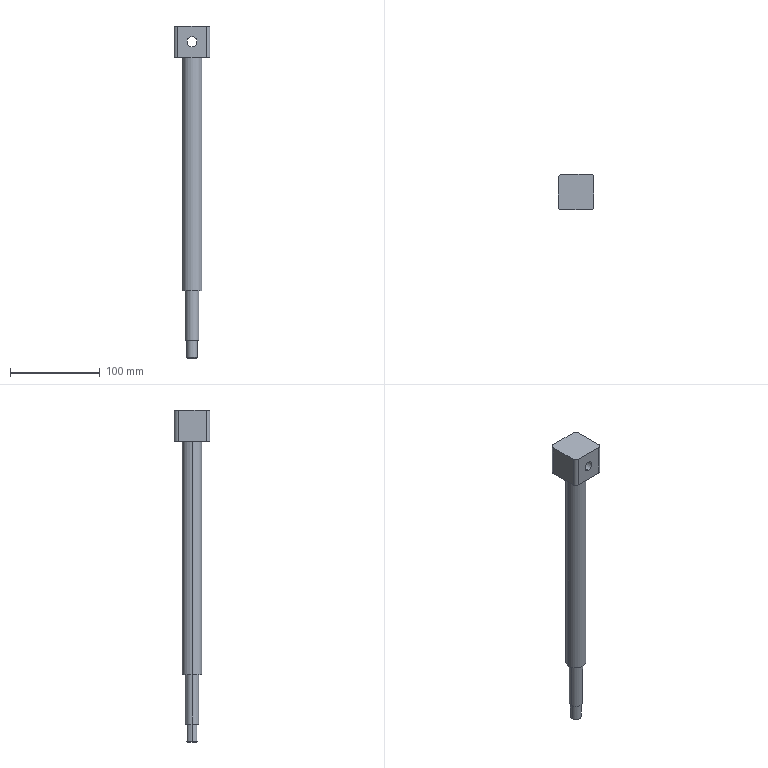Part | SolidWorks | features ICE 4, Chamfer 1, Extrusion 1 | 1 solid | 23 faces | box 40 x 40 x 370 mm | volume 162450 mm3 | cylinder 12 | plane 9 | cone 2 | commonest cylinder face diameters 7.977 x3 11 x2 12 x2 15 x2 22 x2 10 x1
STEP:
#1=CARTESIAN_POINT('',(-5.,0.,-352.5));
#2=VERTEX_POINT('',#1);
#3=CARTESIAN_POINT('',(5.,0.,-352.5));
#4=VERTEX_POINT('',#3);
#5=CARTESIAN_POINT('',(0.,0.,-352.5));
#6=DIRECTION('',(0.,0.,-1.));
#7=DIRECTION('',(-1.,0.,0.));
#8=AXIS2_PLACEMENT_3D('',#5,#6,#7);
#9=CIRCLE('',#8,5.);
#10=EDGE_CURVE('',#2,#4,#9,.T.);
#11=ORIENTED_EDGE('',*,*,#10,.F.);
#12=CARTESIAN_POINT('',(-6.,0.,-351.5));
#13=VERTEX_POINT('',#12);
#14=CARTESIAN_POINT('',(-5.,0.,-352.5));
#15=DIRECTION('',(-0.7071,0.,0.7071));
#16=VECTOR('',#15,1000.);
#17=LINE('',#14,#16);
#18=EDGE_CURVE('',#2,#13,#17,.T.);
#19=ORIENTED_EDGE('',*,*,#18,.T.);
#20=CARTESIAN_POINT('',(6.,0.,-351.5));
#21=VERTEX_POINT('',#20);
#22=CARTESIAN_POINT('',(0.,0.,-351.5));
#23=DIRECTION('',(0.,0.,1.));
#24=DIRECTION('',(-1.,0.,0.));
#25=AXIS2_PLACEMENT_3D('',#22,#23,#24);
#26=CIRCLE('',#25,6.);
#27=EDGE_CURVE('',#21,#13,#26,.T.);
#28=ORIENTED_EDGE('',*,*,#27,.F.);
#29=CARTESIAN_POINT('',(5.,0.,-352.5));
#30=DIRECTION('',(0.7071,0.,0.7071));
#31=VECTOR('',#30,1000.);
#32=LINE('',#29,#31);
#33=EDGE_CURVE('',#4,#21,#32,.T.);
#34=ORIENTED_EDGE('',*,*,#33,.F.);
#35=EDGE_LOOP('',(#11,#19,#28,#34));
#36=FACE_OUTER_BOUND('',#35,.T.);
#37=CARTESIAN_POINT('',(0.,0.,-352.5));
#38=DIRECTION('',(0.,0.,1.));
#39=DIRECTION('',(1.,0.,0.));
#40=AXIS2_PLACEMENT_3D('',#37,#38,#39);
#41=CONICAL_SURFACE('',#40,5.,0.7854);
#42=ADVANCED_FACE('',(#36),#41,.T.);
#43=ORIENTED_EDGE('',*,*,#27,.T.);
#44=CARTESIAN_POINT('',(-6.,0.,-332.5));
#45=VERTEX_POINT('',#44);
#46=CARTESIAN_POINT('',(-6.,0.,-352.5));
#47=DIRECTION('',(0.,0.,1.));
#48=VECTOR('',#47,1000.);
#49=LINE('',#46,#48);
#50=EDGE_CURVE('',#13,#45,#49,.T.);
#51=ORIENTED_EDGE('',*,*,#50,.T.);
#52=CARTESIAN_POINT('',(6.,0.,-332.5));
#53=VERTEX_POINT('',#52);
#54=CARTESIAN_POINT('',(0.,0.,-332.5));
#55=DIRECTION('',(0.,0.,-1.));
#56=DIRECTION('',(-1.,0.,0.));
#57=AXIS2_PLACEMENT_3D('',#54,#55,#56);
#58=CIRCLE('',#57,6.);
#59=EDGE_CURVE('',#45,#53,#58,.T.);
#60=ORIENTED_EDGE('',*,*,#59,.T.);
#61=CARTESIAN_POINT('',(6.,0.,-352.5));
#62=DIRECTION('',(0.,0.,1.));
#63=VECTOR('',#62,1000.);
#64=LINE('',#61,#63);
#65=EDGE_CURVE('',#21,#53,#64,.T.);
#66=ORIENTED_EDGE('',*,*,#65,.F.);
#67=EDGE_LOOP('',(#43,#51,#60,#66));
#68=FACE_OUTER_BOUND('',#67,.T.);
#69=CARTESIAN_POINT('',(0.,0.,-352.5));
#70=DIRECTION('',(0.,0.,1.));
#71=DIRECTION('',(1.,0.,0.));
#72=AXIS2_PLACEMENT_3D('',#69,#70,#71);
#73=CYLINDRICAL_SURFACE('',#72,6.);
#74=ADVANCED_FACE('',(#68),#73,.T.);
#75=CARTESIAN_POINT('',(-7.5,0.,-332.5));
#76=VERTEX_POINT('',#75);
#77=CARTESIAN_POINT('',(7.5,0.,-332.5));
#78=VERTEX_POINT('',#77);
#79=CARTESIAN_POINT('',(0.,0.,-332.5));
#80=DIRECTION('',(0.,0.,-1.));
#81=DIRECTION('',(-1.,0.,0.));
#82=AXIS2_PLACEMENT_3D('',#79,#80,#81);
#83=CIRCLE('',#82,7.5);
#84=EDGE_CURVE('',#76,#78,#83,.T.);
#85=ORIENTED_EDGE('',*,*,#84,.F.);
#86=CARTESIAN_POINT('',(-7.5,0.,-277.5));
#87=VERTEX_POINT('',#86);
#88=CARTESIAN_POINT('',(-7.5,0.,-332.5));
#89=DIRECTION('',(0.,0.,1.));
#90=VECTOR('',#89,1000.);
#91=LINE('',#88,#90);
#92=EDGE_CURVE('',#76,#87,#91,.T.);
#93=ORIENTED_EDGE('',*,*,#92,.T.);
#94=CARTESIAN_POINT('',(7.5,0.,-277.5));
#95=VERTEX_POINT('',#94);
#96=CARTESIAN_POINT('',(0.,0.,-277.5));
#97=DIRECTION('',(0.,0.,-1.));
#98=DIRECTION('',(-1.,0.,0.));
#99=AXIS2_PLACEMENT_3D('',#96,#97,#98);
#100=CIRCLE('',#99,7.5);
#101=EDGE_CURVE('',#87,#95,#100,.T.);
#102=ORIENTED_EDGE('',*,*,#101,.T.);
#103=CARTESIAN_POINT('',(7.5,0.,-332.5));
#104=DIRECTION('',(0.,0.,1.));
#105=VECTOR('',#104,1000.);
#106=LINE('',#103,#105);
#107=EDGE_CURVE('',#78,#95,#106,.T.);
#108=ORIENTED_EDGE('',*,*,#107,.F.);
#109=EDGE_LOOP('',(#85,#93,#102,#108));
#110=FACE_OUTER_BOUND('',#109,.T.);
#111=CARTESIAN_POINT('',(0.,0.,-332.5));
#112=DIRECTION('',(0.,0.,1.));
#113=DIRECTION('',(1.,0.,0.));
#114=AXIS2_PLACEMENT_3D('',#111,#112,#113);
#115=CYLINDRICAL_SURFACE('',#114,7.5);
#116=ADVANCED_FACE('',(#110),#115,.T.);
#117=CARTESIAN_POINT('',(-11.,0.,-277.5));
#118=VERTEX_POINT('',#117);
#119=CARTESIAN_POINT('',(11.,0.,-277.5));
#120=VERTEX_POINT('',#119);
#121=CARTESIAN_POINT('',(0.,0.,-277.5));
#122=DIRECTION('',(0.,0.,-1.));
#123=DIRECTION('',(-1.,0.,0.));
#124=AXIS2_PLACEMENT_3D('',#121,#122,#123);
#125=CIRCLE('',#124,11.);
#126=EDGE_CURVE('',#118,#120,#125,.T.);
#127=ORIENTED_EDGE('',*,*,#126,.F.);
#128=CARTESIAN_POINT('',(-11.,0.,-17.5));
#129=VERTEX_POINT('',#128);
#130=CARTESIAN_POINT('',(-11.,0.,-277.5));
#131=DIRECTION('',(0.,0.,1.));
#132=VECTOR('',#131,1000.);
#133=LINE('',#130,#132);
#134=EDGE_CURVE('',#118,#129,#133,.T.);
#135=ORIENTED_EDGE('',*,*,#134,.T.);
#136=CARTESIAN_POINT('',(11.,0.,-17.5));
#137=VERTEX_POINT('',#136);
#138=CARTESIAN_POINT('',(0.,0.,-17.5));
#139=DIRECTION('',(0.,0.,-1.));
#140=DIRECTION('',(-1.,0.,0.));
#141=AXIS2_PLACEMENT_3D('',#138,#139,#140);
#142=CIRCLE('',#141,11.);
#143=EDGE_CURVE('',#129,#137,#142,.T.);
#144=ORIENTED_EDGE('',*,*,#143,.T.);
#145=CARTESIAN_POINT('',(11.,0.,-277.5));
#146=DIRECTION('',(0.,0.,1.));
#147=VECTOR('',#146,1000.);
#148=LINE('',#145,#147);
#149=EDGE_CURVE('',#120,#137,#148,.T.);
#150=ORIENTED_EDGE('',*,*,#149,.F.);
#151=EDGE_LOOP('',(#127,#135,#144,#150));
#152=FACE_OUTER_BOUND('',#151,.T.);
#153=CARTESIAN_POINT('',(0.,0.,-277.5));
#154=DIRECTION('',(0.,0.,1.));
#155=DIRECTION('',(1.,0.,0.));
#156=AXIS2_PLACEMENT_3D('',#153,#154,#155);
#157=CYLINDRICAL_SURFACE('',#156,11.);
#158=ADVANCED_FACE('',(#152),#157,.T.);
#159=CARTESIAN_POINT('',(0.,-20.,-5.5));
#160=VERTEX_POINT('',#159);
#161=CARTESIAN_POINT('',(0.,-20.,5.5));
#162=VERTEX_POINT('',#161);
#163=CARTESIAN_POINT('',(0.,-20.,0.));
#164=DIRECTION('',(0.,1.,0.));
#165=DIRECTION('',(0.,0.,1.));
#166=AXIS2_PLACEMENT_3D('',#163,#164,#165);
#167=CIRCLE('',#166,5.5);
#168=EDGE_CURVE('',#160,#162,#167,.T.);
#169=ORIENTED_EDGE('',*,*,#168,.F.);
#170=CARTESIAN_POINT('',(0.,20.,-5.5));
#171=VERTEX_POINT('',#170);
#172=CARTESIAN_POINT('',(0.,-34.,-5.5));
#173=DIRECTION('',(0.,1.,0.));
#174=VECTOR('',#173,1000.);
#175=LINE('',#172,#174);
#176=EDGE_CURVE('',#160,#171,#175,.T.);
#177=ORIENTED_EDGE('',*,*,#176,.T.);
#178=CARTESIAN_POINT('',(0.,20.,5.5));
#179=VERTEX_POINT('',#178);
#180=CARTESIAN_POINT('',(0.,20.,0.));
#181=DIRECTION('',(0.,1.,0.));
#182=DIRECTION('',(0.,0.,1.));
#183=AXIS2_PLACEMENT_3D('',#180,#181,#182);
#184=CIRCLE('',#183,5.5);
#185=EDGE_CURVE('',#171,#179,#184,.T.);
#186=ORIENTED_EDGE('',*,*,#185,.T.);
#187=CARTESIAN_POINT('',(0.,-34.,5.5));
#188=DIRECTION('',(0.,1.,0.));
#189=VECTOR('',#188,1000.);
#190=LINE('',#187,#189);
#191=EDGE_CURVE('',#162,#179,#190,.T.);
#192=ORIENTED_EDGE('',*,*,#191,.F.);
#193=EDGE_LOOP('',(#169,#177,#186,#192));
#194=FACE_OUTER_BOUND('',#193,.T.);
#195=CARTESIAN_POINT('',(0.,-34.,0.));
#196=DIRECTION('',(0.,1.,0.));
#197=DIRECTION('',(0.,0.,1.));
#198=AXIS2_PLACEMENT_3D('',#195,#196,#197);
#199=CYLINDRICAL_SURFACE('',#198,5.5);
#200=ADVANCED_FACE('',(#194),#199,.F.);
#201=CARTESIAN_POINT('',(0.,0.,-332.5));
#202=DIRECTION('',(0.,0.,-1.));
#203=DIRECTION('',(-1.,0.,0.));
#204=AXIS2_PLACEMENT_3D('',#201,#202,#203);
#205=CIRCLE('',#204,7.5);
#206=EDGE_CURVE('',#78,#76,#205,.T.);
#207=ORIENTED_EDGE('',*,*,#206,.T.);
#208=ORIENTED_EDGE('',*,*,#84,.T.);
#209=EDGE_LOOP('',(#207,#208));
#210=FACE_OUTER_BOUND('',#209,.T.);
#211=CARTESIAN_POINT('',(0.,0.,-332.5));
#212=DIRECTION('',(0.,0.,-1.));
#213=DIRECTION('',(-1.,0.,0.));
#214=AXIS2_PLACEMENT_3D('',#211,#212,#213);
#215=CIRCLE('',#214,6.);
#216=EDGE_CURVE('',#53,#45,#215,.T.);
#217=ORIENTED_EDGE('',*,*,#216,.F.);
#218=ORIENTED_EDGE('',*,*,#59,.F.);
#219=EDGE_LOOP('',(#217,#218));
#220=FACE_BOUND('',#219,.T.);
#221=CARTESIAN_POINT('',(0.,0.,-332.5));
#222=DIRECTION('',(0.,0.,-1.));
#223=DIRECTION('',(-1.,0.,0.));
#224=AXIS2_PLACEMENT_3D('',#221,#222,#223);
#225=PLANE('',#224);
#226=ADVANCED_FACE('',(#210,#220),#225,.T.);
#227=CARTESIAN_POINT('',(0.,0.,-277.5));
#228=DIRECTION('',(0.,0.,-1.));
#229=DIRECTION('',(-1.,0.,0.));
#230=AXIS2_PLACEMENT_3D('',#227,#228,#229);
#231=CIRCLE('',#230,11.);
#232=EDGE_CURVE('',#120,#118,#231,.T.);
#233=ORIENTED_EDGE('',*,*,#232,.T.);
#234=ORIENTED_EDGE('',*,*,#126,.T.);
#235=EDGE_LOOP('',(#233,#234));
#236=FACE_OUTER_BOUND('',#235,.T.);
#237=CARTESIAN_POINT('',(0.,0.,-277.5));
#238=DIRECTION('',(0.,0.,-1.));
#239=DIRECTION('',(-1.,0.,0.));
#240=AXIS2_PLACEMENT_3D('',#237,#238,#239);
#241=CIRCLE('',#240,7.5);
#242=EDGE_CURVE('',#95,#87,#241,.T.);
#243=ORIENTED_EDGE('',*,*,#242,.F.);
#244=ORIENTED_EDGE('',*,*,#101,.F.);
#245=EDGE_LOOP('',(#243,#244));
#246=FACE_BOUND('',#245,.T.);
#247=CARTESIAN_POINT('',(0.,0.,-277.5));
#248=DIRECTION('',(0.,0.,-1.));
#249=DIRECTION('',(-1.,0.,0.));
#250=AXIS2_PLACEMENT_3D('',#247,#248,#249);
#251=PLANE('',#250);
#252=ADVANCED_FACE('',(#236,#246),#251,.T.);
#253=CARTESIAN_POINT('',(-15.,20.,-17.5));
#254=VERTEX_POINT('',#253);
#255=CARTESIAN_POINT('',(-20.,15.,-17.5));
#256=VERTEX_POINT('',#255);
#257=CARTESIAN_POINT('',(-15.,15.,-17.5));
#258=DIRECTION('',(0.,0.,1.));
#259=DIRECTION('',(-1.,0.,0.));
#260=AXIS2_PLACEMENT_3D('',#257,#258,#259);
#261=CIRCLE('',#260,5.);
#262=EDGE_CURVE('',#254,#256,#261,.T.);
#263=ORIENTED_EDGE('',*,*,#262,.F.);
#264=CARTESIAN_POINT('',(16.011,20.,-17.5));
#265=VERTEX_POINT('',#264);
#266=CARTESIAN_POINT('',(-15.,20.,-17.5));
#267=DIRECTION('',(-1.,0.,0.));
#268=VECTOR('',#267,1000.);
#269=LINE('',#266,#268);
#270=EDGE_CURVE('',#265,#254,#269,.T.);
#271=ORIENTED_EDGE('',*,*,#270,.F.);
#272=CARTESIAN_POINT('',(20.,16.011,-17.5));
#273=VERTEX_POINT('',#272);
#274=CARTESIAN_POINT('',(16.011,16.011,-17.5));
#275=DIRECTION('',(0.,0.,1.));
#276=DIRECTION('',(1.,0.,0.));
#277=AXIS2_PLACEMENT_3D('',#274,#275,#276);
#278=CIRCLE('',#277,3.989);
#279=EDGE_CURVE('',#273,#265,#278,.T.);
#280=ORIENTED_EDGE('',*,*,#279,.F.);
#281=CARTESIAN_POINT('',(20.,-16.011,-17.5));
#282=VERTEX_POINT('',#281);
#283=CARTESIAN_POINT('',(20.,16.011,-17.5));
#284=DIRECTION('',(0.,1.,0.));
#285=VECTOR('',#284,1000.);
#286=LINE('',#283,#285);
#287=EDGE_CURVE('',#282,#273,#286,.T.);
#288=ORIENTED_EDGE('',*,*,#287,.F.);
#289=CARTESIAN_POINT('',(16.011,-20.,-17.5));
#290=VERTEX_POINT('',#289);
#291=CARTESIAN_POINT('',(16.011,-16.011,-17.5));
#292=DIRECTION('',(0.,0.,1.));
#293=DIRECTION('',(1.,0.,0.));
#294=AXIS2_PLACEMENT_3D('',#291,#292,#293);
#295=CIRCLE('',#294,3.989);
#296=EDGE_CURVE('',#290,#282,#295,.T.);
#297=ORIENTED_EDGE('',*,*,#296,.F.);
#298=CARTESIAN_POINT('',(-16.011,-20.,-17.5));
#299=VERTEX_POINT('',#298);
#300=CARTESIAN_POINT('',(-16.011,-20.,-17.5));
#301=DIRECTION('',(1.,0.,0.));
#302=VECTOR('',#301,1000.);
#303=LINE('',#300,#302);
#304=EDGE_CURVE('',#299,#290,#303,.T.);
#305=ORIENTED_EDGE('',*,*,#304,.F.);
#306=CARTESIAN_POINT('',(-20.,-16.011,-17.5));
#307=VERTEX_POINT('',#306);
#308=CARTESIAN_POINT('',(-16.011,-16.011,-17.5));
#309=DIRECTION('',(0.,0.,1.));
#310=DIRECTION('',(-1.,0.,0.));
#311=AXIS2_PLACEMENT_3D('',#308,#309,#310);
#312=CIRCLE('',#311,3.989);
#313=EDGE_CURVE('',#307,#299,#312,.T.);
#314=ORIENTED_EDGE('',*,*,#313,.F.);
#315=CARTESIAN_POINT('',(-20.,15.,-17.5));
#316=DIRECTION('',(0.,-1.,0.));
#317=VECTOR('',#316,1000.);
#318=LINE('',#315,#317);
#319=EDGE_CURVE('',#256,#307,#318,.T.);
#320=ORIENTED_EDGE('',*,*,#319,.F.);
#321=EDGE_LOOP('',(#263,#271,#280,#288,#297,#305,#314,#320));
#322=FACE_OUTER_BOUND('',#321,.T.);
#323=CARTESIAN_POINT('',(0.,0.,-17.5));
#324=DIRECTION('',(0.,0.,-1.));
#325=DIRECTION('',(-1.,0.,0.));
#326=AXIS2_PLACEMENT_3D('',#323,#324,#325);
#327=CIRCLE('',#326,11.);
#328=EDGE_CURVE('',#137,#129,#327,.T.);
#329=ORIENTED_EDGE('',*,*,#328,.F.);
#330=ORIENTED_EDGE('',*,*,#143,.F.);
#331=EDGE_LOOP('',(#329,#330));
#332=FACE_BOUND('',#331,.T.);
#333=CARTESIAN_POINT('',(-15.,15.,-17.5));
#334=DIRECTION('',(0.,0.,-1.));
#335=DIRECTION('',(-1.,0.,0.));
#336=AXIS2_PLACEMENT_3D('',#333,#334,#335);
#337=PLANE('',#336);
#338=ADVANCED_FACE('',(#322,#332),#337,.T.);
#339=ORIENTED_EDGE('',*,*,#262,.T.);
#340=CARTESIAN_POINT('',(-20.,15.,17.5));
#341=VERTEX_POINT('',#340);
#342=CARTESIAN_POINT('',(-20.,15.,17.5));
#343=DIRECTION('',(0.,0.,-1.));
#344=VECTOR('',#343,1000.);
#345=LINE('',#342,#344);
#346=EDGE_CURVE('',#341,#256,#345,.T.);
#347=ORIENTED_EDGE('',*,*,#346,.F.);
#348=CARTESIAN_POINT('',(-15.,20.,17.5));
#349=VERTEX_POINT('',#348);
#350=CARTESIAN_POINT('',(-15.,15.,17.5));
#351=DIRECTION('',(0.,0.,1.));
#352=DIRECTION('',(-1.,0.,0.));
#353=AXIS2_PLACEMENT_3D('',#350,#351,#352);
#354=CIRCLE('',#353,5.);
#355=EDGE_CURVE('',#349,#341,#354,.T.);
#356=ORIENTED_EDGE('',*,*,#355,.F.);
#357=CARTESIAN_POINT('',(-15.,20.,17.5));
#358=DIRECTION('',(0.,0.,-1.));
#359=VECTOR('',#358,1000.);
#360=LINE('',#357,#359);
#361=EDGE_CURVE('',#349,#254,#360,.T.);
#362=ORIENTED_EDGE('',*,*,#361,.T.);
#363=EDGE_LOOP('',(#339,#347,#356,#362));
#364=FACE_OUTER_BOUND('',#363,.T.);
#365=CARTESIAN_POINT('',(-15.,15.,17.5));
#366=DIRECTION('',(0.,0.,-1.));
#367=DIRECTION('',(-1.,0.,0.));
#368=AXIS2_PLACEMENT_3D('',#365,#366,#367);
#369=CYLINDRICAL_SURFACE('',#368,5.);
#370=ADVANCED_FACE('',(#364),#369,.T.);
#371=ORIENTED_EDGE('',*,*,#319,.T.);
#372=CARTESIAN_POINT('',(-20.,-16.011,17.5));
#373=VERTEX_POINT('',#372);
#374=CARTESIAN_POINT('',(-20.,-16.011,17.5));
#375=DIRECTION('',(0.,0.,-1.));
#376=VECTOR('',#375,1000.);
#377=LINE('',#374,#376);
#378=EDGE_CURVE('',#373,#307,#377,.T.);
#379=ORIENTED_EDGE('',*,*,#378,.F.);
#380=CARTESIAN_POINT('',(-20.,15.,17.5));
#381=DIRECTION('',(0.,-1.,0.));
#382=VECTOR('',#381,1000.);
#383=LINE('',#380,#382);
#384=EDGE_CURVE('',#341,#373,#383,.T.);
#385=ORIENTED_EDGE('',*,*,#384,.F.);
#386=ORIENTED_EDGE('',*,*,#346,.T.);
#387=EDGE_LOOP('',(#371,#379,#385,#386));
#388=FACE_OUTER_BOUND('',#387,.T.);
#389=CARTESIAN_POINT('',(-20.,15.,17.5));
#390=DIRECTION('',(1.,0.,0.));
#391=DIRECTION('',(0.,1.,0.));
#392=AXIS2_PLACEMENT_3D('',#389,#390,#391);
#393=PLANE('',#392);
#394=ADVANCED_FACE('',(#388),#393,.F.);
#395=ORIENTED_EDGE('',*,*,#313,.T.);
#396=CARTESIAN_POINT('',(-16.011,-20.,17.5));
#397=VERTEX_POINT('',#396);
#398=CARTESIAN_POINT('',(-16.011,-20.,17.5));
#399=DIRECTION('',(0.,0.,-1.));
#400=VECTOR('',#399,1000.);
#401=LINE('',#398,#400);
#402=EDGE_CURVE('',#397,#299,#401,.T.);
#403=ORIENTED_EDGE('',*,*,#402,.F.);
#404=CARTESIAN_POINT('',(-16.011,-16.011,17.5));
#405=DIRECTION('',(0.,0.,1.));
#406=DIRECTION('',(-1.,0.,0.));
#407=AXIS2_PLACEMENT_3D('',#404,#405,#406);
#408=CIRCLE('',#407,3.989);
#409=EDGE_CURVE('',#373,#397,#408,.T.);
#410=ORIENTED_EDGE('',*,*,#409,.F.);
#411=ORIENTED_EDGE('',*,*,#378,.T.);
#412=EDGE_LOOP('',(#395,#403,#410,#411));
#413=FACE_OUTER_BOUND('',#412,.T.);
#414=CARTESIAN_POINT('',(-16.011,-16.011,17.5));
#415=DIRECTION('',(0.,0.,-1.));
#416=DIRECTION('',(-1.,0.,0.));
#417=AXIS2_PLACEMENT_3D('',#414,#415,#416);
#418=CYLINDRICAL_SURFACE('',#417,3.989);
#419=ADVANCED_FACE('',(#413),#418,.T.);
#420=CARTESIAN_POINT('',(0.,-20.,0.));
#421=DIRECTION('',(0.,1.,0.));
#422=DIRECTION('',(0.,0.,1.));
#423=AXIS2_PLACEMENT_3D('',#420,#421,#422);
#424=CIRCLE('',#423,5.5);
#425=EDGE_CURVE('',#162,#160,#424,.T.);
#426=ORIENTED_EDGE('',*,*,#425,.T.);
#427=ORIENTED_EDGE('',*,*,#168,.T.);
#428=EDGE_LOOP('',(#426,#427));
#429=FACE_BOUND('',#428,.T.);
#430=ORIENTED_EDGE('',*,*,#304,.T.);
#431=CARTESIAN_POINT('',(16.011,-20.,17.5));
#432=VERTEX_POINT('',#431);
#433=CARTESIAN_POINT('',(16.011,-20.,17.5));
#434=DIRECTION('',(0.,0.,-1.));
#435=VECTOR('',#434,1000.);
#436=LINE('',#433,#435);
#437=EDGE_CURVE('',#432,#290,#436,.T.);
#438=ORIENTED_EDGE('',*,*,#437,.F.);
#439=CARTESIAN_POINT('',(-16.011,-20.,17.5));
#440=DIRECTION('',(1.,0.,0.));
#441=VECTOR('',#440,1000.);
#442=LINE('',#439,#441);
#443=EDGE_CURVE('',#397,#432,#442,.T.);
#444=ORIENTED_EDGE('',*,*,#443,.F.);
#445=ORIENTED_EDGE('',*,*,#402,.T.);
#446=EDGE_LOOP('',(#430,#438,#444,#445));
#447=FACE_OUTER_BOUND('',#446,.T.);
#448=CARTESIAN_POINT('',(-16.011,-20.,17.5));
#449=DIRECTION('',(0.,1.,0.));
#450=DIRECTION('',(0.,0.,1.));
#451=AXIS2_PLACEMENT_3D('',#448,#449,#450);
#452=PLANE('',#451);
#453=ADVANCED_FACE('',(#429,#447),#452,.F.);
#454=ORIENTED_EDGE('',*,*,#296,.T.);
#455=CARTESIAN_POINT('',(20.,-16.011,17.5));
#456=VERTEX_POINT('',#455);
#457=CARTESIAN_POINT('',(20.,-16.011,17.5));
#458=DIRECTION('',(0.,0.,-1.));
#459=VECTOR('',#458,1000.);
#460=LINE('',#457,#459);
#461=EDGE_CURVE('',#456,#282,#460,.T.);
#462=ORIENTED_EDGE('',*,*,#461,.F.);
#463=CARTESIAN_POINT('',(16.011,-16.011,17.5));
#464=DIRECTION('',(0.,0.,1.));
#465=DIRECTION('',(1.,0.,0.));
#466=AXIS2_PLACEMENT_3D('',#463,#464,#465);
#467=CIRCLE('',#466,3.989);
#468=EDGE_CURVE('',#432,#456,#467,.T.);
#469=ORIENTED_EDGE('',*,*,#468,.F.);
#470=ORIENTED_EDGE('',*,*,#437,.T.);
#471=EDGE_LOOP('',(#454,#462,#469,#470));
#472=FACE_OUTER_BOUND('',#471,.T.);
#473=CARTESIAN_POINT('',(16.011,-16.011,17.5));
#474=DIRECTION('',(0.,0.,-1.));
#475=DIRECTION('',(-1.,0.,0.));
#476=AXIS2_PLACEMENT_3D('',#473,#474,#475);
#477=CYLINDRICAL_SURFACE('',#476,3.989);
#478=ADVANCED_FACE('',(#472),#477,.T.);
#479=ORIENTED_EDGE('',*,*,#287,.T.);
#480=CARTESIAN_POINT('',(20.,16.011,17.5));
#481=VERTEX_POINT('',#480);
#482=CARTESIAN_POINT('',(20.,16.011,17.5));
#483=DIRECTION('',(0.,0.,-1.));
#484=VECTOR('',#483,1000.);
#485=LINE('',#482,#484);
#486=EDGE_CURVE('',#481,#273,#485,.T.);
#487=ORIENTED_EDGE('',*,*,#486,.F.);
#488=CARTESIAN_POINT('',(20.,16.011,17.5));
#489=DIRECTION('',(0.,1.,0.));
#490=VECTOR('',#489,1000.);
#491=LINE('',#488,#490);
#492=EDGE_CURVE('',#456,#481,#491,.T.);
#493=ORIENTED_EDGE('',*,*,#492,.F.);
#494=ORIENTED_EDGE('',*,*,#461,.T.);
#495=EDGE_LOOP('',(#479,#487,#493,#494));
#496=FACE_OUTER_BOUND('',#495,.T.);
#497=CARTESIAN_POINT('',(20.,16.011,17.5));
#498=DIRECTION('',(-1.,0.,0.));
#499=DIRECTION('',(0.,-1.,0.));
#500=AXIS2_PLACEMENT_3D('',#497,#498,#499);
#501=PLANE('',#500);
#502=ADVANCED_FACE('',(#496),#501,.F.);
#503=ORIENTED_EDGE('',*,*,#279,.T.);
#504=CARTESIAN_POINT('',(16.011,20.,17.5));
#505=VERTEX_POINT('',#504);
#506=CARTESIAN_POINT('',(16.011,20.,17.5));
#507=DIRECTION('',(0.,0.,-1.));
#508=VECTOR('',#507,1000.);
#509=LINE('',#506,#508);
#510=EDGE_CURVE('',#505,#265,#509,.T.);
#511=ORIENTED_EDGE('',*,*,#510,.F.);
#512=CARTESIAN_POINT('',(16.011,16.011,17.5));
#513=DIRECTION('',(0.,0.,1.));
#514=DIRECTION('',(1.,0.,0.));
#515=AXIS2_PLACEMENT_3D('',#512,#513,#514);
#516=CIRCLE('',#515,3.989);
#517=EDGE_CURVE('',#481,#505,#516,.T.);
#518=ORIENTED_EDGE('',*,*,#517,.F.);
#519=ORIENTED_EDGE('',*,*,#486,.T.);
#520=EDGE_LOOP('',(#503,#511,#518,#519));
#521=FACE_OUTER_BOUND('',#520,.T.);
#522=CARTESIAN_POINT('',(16.011,16.011,17.5));
#523=DIRECTION('',(0.,0.,-1.));
#524=DIRECTION('',(-1.,0.,0.));
#525=AXIS2_PLACEMENT_3D('',#522,#523,#524);
#526=CYLINDRICAL_SURFACE('',#525,3.989);
#527=ADVANCED_FACE('',(#521),#526,.T.);
#528=CARTESIAN_POINT('',(0.,20.,0.));
#529=DIRECTION('',(0.,1.,0.));
#530=DIRECTION('',(0.,0.,1.));
#531=AXIS2_PLACEMENT_3D('',#528,#529,#530);
#532=CIRCLE('',#531,5.5);
#533=EDGE_CURVE('',#179,#171,#532,.T.);
#534=ORIENTED_EDGE('',*,*,#533,.F.);
#535=ORIENTED_EDGE('',*,*,#185,.F.);
#536=EDGE_LOOP('',(#534,#535));
#537=FACE_BOUND('',#536,.T.);
#538=ORIENTED_EDGE('',*,*,#270,.T.);
#539=ORIENTED_EDGE('',*,*,#361,.F.);
#540=CARTESIAN_POINT('',(-15.,20.,17.5));
#541=DIRECTION('',(-1.,0.,0.));
#542=VECTOR('',#541,1000.);
#543=LINE('',#540,#542);
#544=EDGE_CURVE('',#505,#349,#543,.T.);
#545=ORIENTED_EDGE('',*,*,#544,.F.);
#546=ORIENTED_EDGE('',*,*,#510,.T.);
#547=EDGE_LOOP('',(#538,#539,#545,#546));
#548=FACE_OUTER_BOUND('',#547,.T.);
#549=CARTESIAN_POINT('',(-15.,20.,17.5));
#550=DIRECTION('',(0.,-1.,0.));
#551=DIRECTION('',(0.,0.,-1.));
#552=AXIS2_PLACEMENT_3D('',#549,#550,#551);
#553=PLANE('',#552);
#554=ADVANCED_FACE('',(#537,#548),#553,.F.);
#555=ORIENTED_EDGE('',*,*,#355,.T.);
#556=ORIENTED_EDGE('',*,*,#384,.T.);
#557=ORIENTED_EDGE('',*,*,#409,.T.);
#558=ORIENTED_EDGE('',*,*,#443,.T.);
#559=ORIENTED_EDGE('',*,*,#468,.T.);
#560=ORIENTED_EDGE('',*,*,#492,.T.);
#561=ORIENTED_EDGE('',*,*,#517,.T.);
#562=ORIENTED_EDGE('',*,*,#544,.T.);
#563=EDGE_LOOP('',(#555,#556,#557,#558,#559,#560,#561,#562));
#564=FACE_OUTER_BOUND('',#563,.T.);
#565=CARTESIAN_POINT('',(-15.,15.,17.5));
#566=DIRECTION('',(0.,0.,-1.));
#567=DIRECTION('',(-1.,0.,0.));
#568=AXIS2_PLACEMENT_3D('',#565,#566,#567);
#569=PLANE('',#568);
#570=ADVANCED_FACE('',(#564),#569,.F.);
#571=ORIENTED_EDGE('',*,*,#176,.F.);
#572=ORIENTED_EDGE('',*,*,#425,.F.);
#573=ORIENTED_EDGE('',*,*,#191,.T.);
#574=ORIENTED_EDGE('',*,*,#533,.T.);
#575=EDGE_LOOP('',(#571,#572,#573,#574));
#576=FACE_OUTER_BOUND('',#575,.T.);
#577=CARTESIAN_POINT('',(0.,-34.,0.));
#578=DIRECTION('',(0.,1.,0.));
#579=DIRECTION('',(0.,0.,1.));
#580=AXIS2_PLACEMENT_3D('',#577,#578,#579);
#581=CYLINDRICAL_SURFACE('',#580,5.5);
#582=ADVANCED_FACE('',(#576),#581,.F.);
#583=ORIENTED_EDGE('',*,*,#134,.F.);
#584=ORIENTED_EDGE('',*,*,#232,.F.);
#585=ORIENTED_EDGE('',*,*,#149,.T.);
#586=ORIENTED_EDGE('',*,*,#328,.T.);
#587=EDGE_LOOP('',(#583,#584,#585,#586));
#588=FACE_OUTER_BOUND('',#587,.T.);
#589=CARTESIAN_POINT('',(0.,0.,-277.5));
#590=DIRECTION('',(0.,0.,1.));
#591=DIRECTION('',(1.,0.,0.));
#592=AXIS2_PLACEMENT_3D('',#589,#590,#591);
#593=CYLINDRICAL_SURFACE('',#592,11.);
#594=ADVANCED_FACE('',(#588),#593,.T.);
#595=ORIENTED_EDGE('',*,*,#92,.F.);
#596=ORIENTED_EDGE('',*,*,#206,.F.);
#597=ORIENTED_EDGE('',*,*,#107,.T.);
#598=ORIENTED_EDGE('',*,*,#242,.T.);
#599=EDGE_LOOP('',(#595,#596,#597,#598));
#600=FACE_OUTER_BOUND('',#599,.T.);
#601=CARTESIAN_POINT('',(0.,0.,-332.5));
#602=DIRECTION('',(0.,0.,1.));
#603=DIRECTION('',(1.,0.,0.));
#604=AXIS2_PLACEMENT_3D('',#601,#602,#603);
#605=CYLINDRICAL_SURFACE('',#604,7.5);
#606=ADVANCED_FACE('',(#600),#605,.T.);
#607=ORIENTED_EDGE('',*,*,#50,.F.);
#608=CARTESIAN_POINT('',(0.,0.,-351.5));
#609=DIRECTION('',(0.,0.,1.));
#610=DIRECTION('',(-1.,0.,0.));
#611=AXIS2_PLACEMENT_3D('',#608,#609,#610);
#612=CIRCLE('',#611,6.);
#613=EDGE_CURVE('',#13,#21,#612,.T.);
#614=ORIENTED_EDGE('',*,*,#613,.T.);
#615=ORIENTED_EDGE('',*,*,#65,.T.);
#616=ORIENTED_EDGE('',*,*,#216,.T.);
#617=EDGE_LOOP('',(#607,#614,#615,#616));
#618=FACE_OUTER_BOUND('',#617,.T.);
#619=CARTESIAN_POINT('',(0.,0.,-352.5));
#620=DIRECTION('',(0.,0.,1.));
#621=DIRECTION('',(1.,0.,0.));
#622=AXIS2_PLACEMENT_3D('',#619,#620,#621);
#623=CYLINDRICAL_SURFACE('',#622,6.);
#624=ADVANCED_FACE('',(#618),#623,.T.);
#625=CARTESIAN_POINT('',(0.,0.,-352.5));
#626=DIRECTION('',(0.,0.,-1.));
#627=DIRECTION('',(-1.,0.,0.));
#628=AXIS2_PLACEMENT_3D('',#625,#626,#627);
#629=CIRCLE('',#628,5.);
#630=EDGE_CURVE('',#4,#2,#629,.T.);
#631=ORIENTED_EDGE('',*,*,#630,.T.);
#632=ORIENTED_EDGE('',*,*,#10,.T.);
#633=EDGE_LOOP('',(#631,#632));
#634=FACE_OUTER_BOUND('',#633,.T.);
#635=CARTESIAN_POINT('',(0.,0.,-352.5));
#636=DIRECTION('',(0.,0.,-1.));
#637=DIRECTION('',(-1.,0.,0.));
#638=AXIS2_PLACEMENT_3D('',#635,#636,#637);
#639=PLANE('',#638);
#640=ADVANCED_FACE('',(#634),#639,.T.);
#641=ORIENTED_EDGE('',*,*,#18,.F.);
#642=ORIENTED_EDGE('',*,*,#630,.F.);
#643=ORIENTED_EDGE('',*,*,#33,.T.);
#644=ORIENTED_EDGE('',*,*,#613,.F.);
#645=EDGE_LOOP('',(#641,#642,#643,#644));
#646=FACE_OUTER_BOUND('',#645,.T.);
#647=CARTESIAN_POINT('',(0.,0.,-352.5));
#648=DIRECTION('',(0.,0.,1.));
#649=DIRECTION('',(1.,0.,0.));
#650=AXIS2_PLACEMENT_3D('',#647,#648,#649);
#651=CONICAL_SURFACE('',#650,5.,0.7854);
#652=ADVANCED_FACE('',(#646),#651,.T.);
#653=CLOSED_SHELL('',(#42,#74,#116,#158,#200,#226,#252,#338,#370,#394,#419,#453,#478,#502,#527,#554,#570,#582,#594,#606,#624,#640,#652));
#654=MANIFOLD_SOLID_BREP('',#653);
#655=CARTESIAN_POINT('',(0.,0.,0.));
#656=DIRECTION('',(0.,0.,1.));
#657=DIRECTION('',(1.,0.,0.));
#658=AXIS2_PLACEMENT_3D('',#655,#656,#657);
#659=(LENGTH_UNIT()NAMED_UNIT(*)SI_UNIT(.MILLI.,.METRE.));
#660=UNCERTAINTY_MEASURE_WITH_UNIT(LENGTH_MEASURE(0.00001),#659,'','');
#661=(NAMED_UNIT(*)PLANE_ANGLE_UNIT()SI_UNIT($,.RADIAN.));
#662=(NAMED_UNIT(*)SI_UNIT($,.STERADIAN.)SOLID_ANGLE_UNIT());
#663=(GEOMETRIC_REPRESENTATION_CONTEXT(3)GLOBAL_UNCERTAINTY_ASSIGNED_CONTEXT((#660))GLOBAL_UNIT_ASSIGNED_CONTEXT((#659,#661,#662))REPRESENTATION_CONTEXT('',''));
#664=ADVANCED_BREP_SHAPE_REPRESENTATION('',(#654,#658),#663);